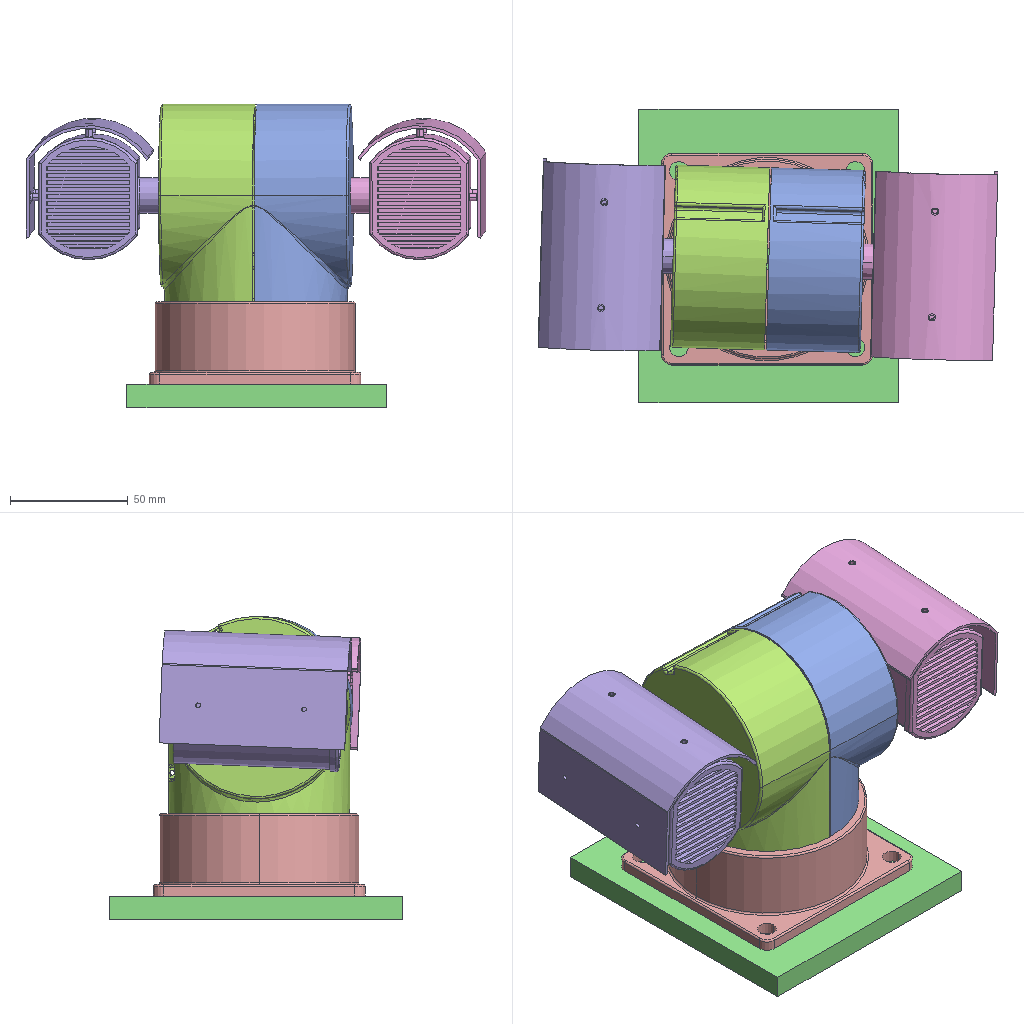Assembly | SolidWorks | 5 different items | 5 placed | box 195 x 125 x 129 mm
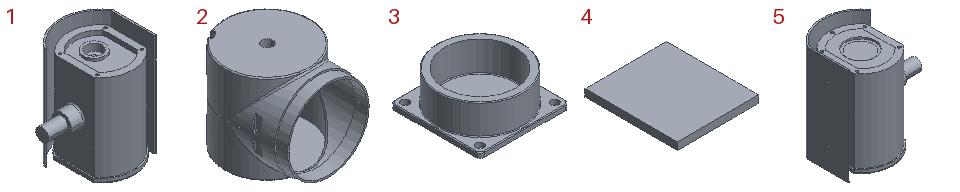Parts list (item | quantity | size | volume | features):
1 | x1 | 71.25 x 57.25 x 79 mm | 129826 mm3 | features ICE 14, Dome 1, Extrusion 1, Fillet 1, Scale 1
2 | x1 | 77.5 x 94 x 80.75 mm | 41607 mm3 | features ICE 7, Fillet 4, Extrusion 1, MirrorSolid 1, Scale 1, Shell 1
3 | x1 | 90 x 90 x 35 mm | 90534 mm3 | features ICE 4, Extrusion 1, Fillet 1, Scale 1
4 | x1 | 110.487 x 124.868 x 10 mm | 137963 mm3 | features Extrusion 1
5 | x1 | 71.25 x 57.25 x 79 mm | 131185 mm3 | features ICE 17, Dome 1, Extrusion 1, Fillet 1, MirrorSolid 1, Scale 1
Mates (type | each side: item.copy, entity, surface, feature):
Concentric | 3.1 face cylinder Cut-Extrude1 | 2.1 face cylinder Boss-Extrude3
Coincident | 3.1 face plane Boss-Extrude2 | 2.1 face plane Mirror2
Concentric | 2.1 face cylinder Cut-Extrude1 | 1.1 face cylinder Boss-Extrude7
Coincident | 2.1 face plane Boss-Extrude1 | 1.1 face plane Boss-Extrude8
Concentric | 2.1 face cylinder Mirror2 | 5.1 face cylinder Boss-Extrude9
Coincident | 2.1 face plane Mirror2 | 5.1 face plane Boss-Extrude10
Coincident | 5.1 face plane Mirror2 | 1.1 face plane Boss-Extrude2